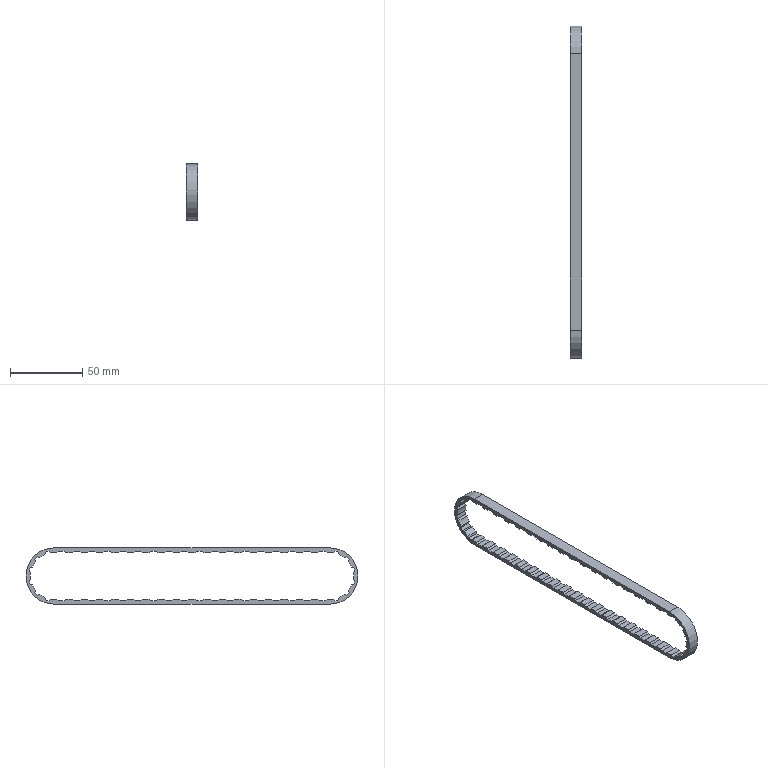Part | NX | features CPROJ 5, DATUM_CSYS 4, EXTRUDE 3, SKETCH 3, EXTRACT_BODY 2, TRIM BODY 2, Container 1, Delete Body 1, Geometry Instance 1, Pattern Geometry 1, UNITE 1 | 1 solid | 198 faces | box 8 x 230.5 x 39 mm | volume 11364 mm3 | plane 170 | cylinder 28 | commonest cylinder face diameters 32.525 x14 35 x12 39 x2